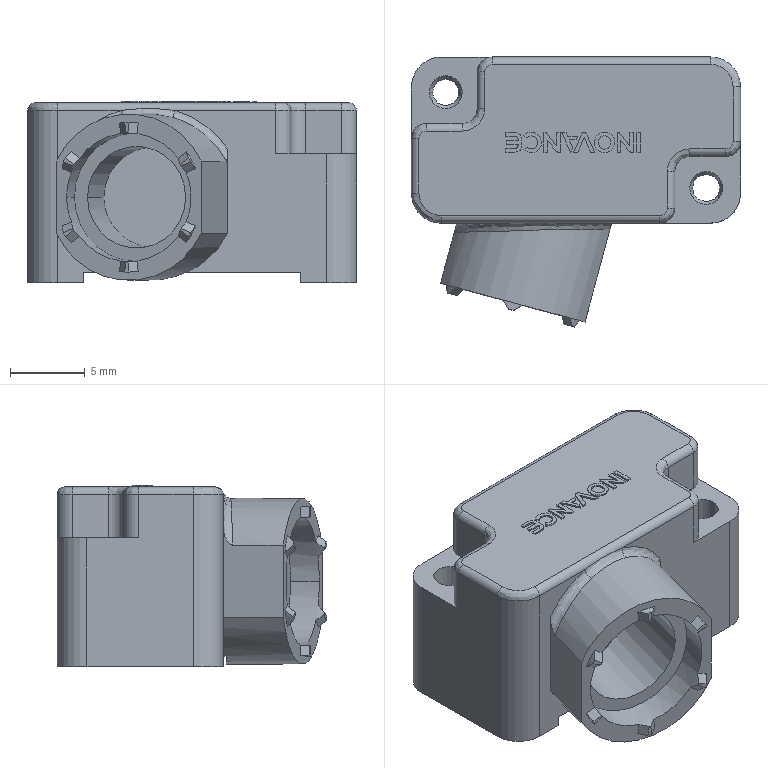Part | STEP file | 21E8-005-1073-P4_1_1_1_1_2 | 1 solid | 252 faces | box 22 x 18.036 x 12.1 mm | volume 1630 mm3 | plane 157 | cylinder 60 | spline 35 | commonest cylinder face diameters 1 x20 2.2 x8 2 x6 10 x6 0.4 x4 3 x4